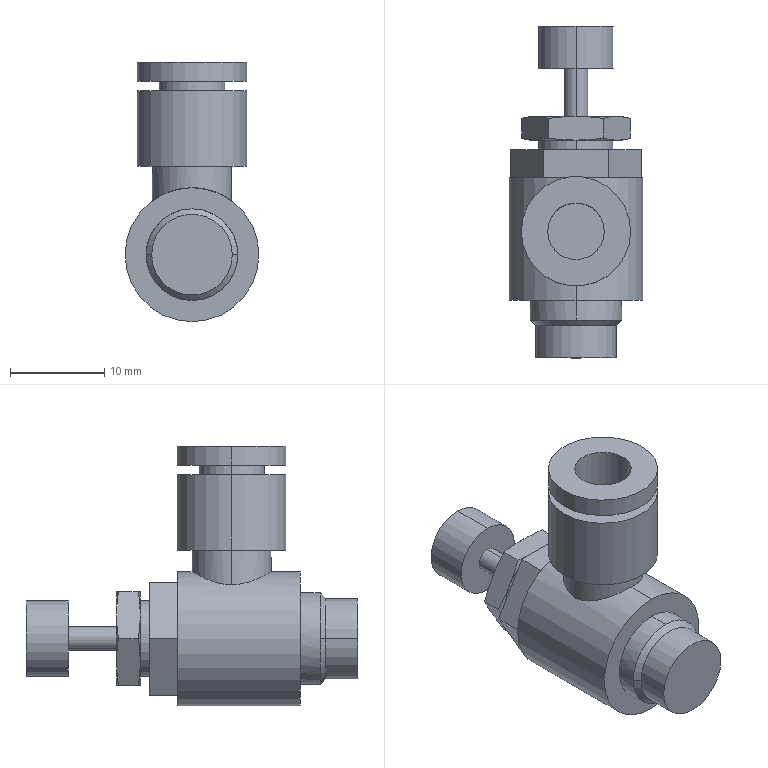Part | STEP file | AS2201FG-01-06S | 1 solid | 61 faces | box 14.2 x 35.2 x 27.5 mm | volume 4200 mm3 | plane 25 | cylinder 22 | cone 14 | commonest cylinder face diameters 8 x4 11.6 x4 2.5 x2 6 x2 7 x2 8.4 x2